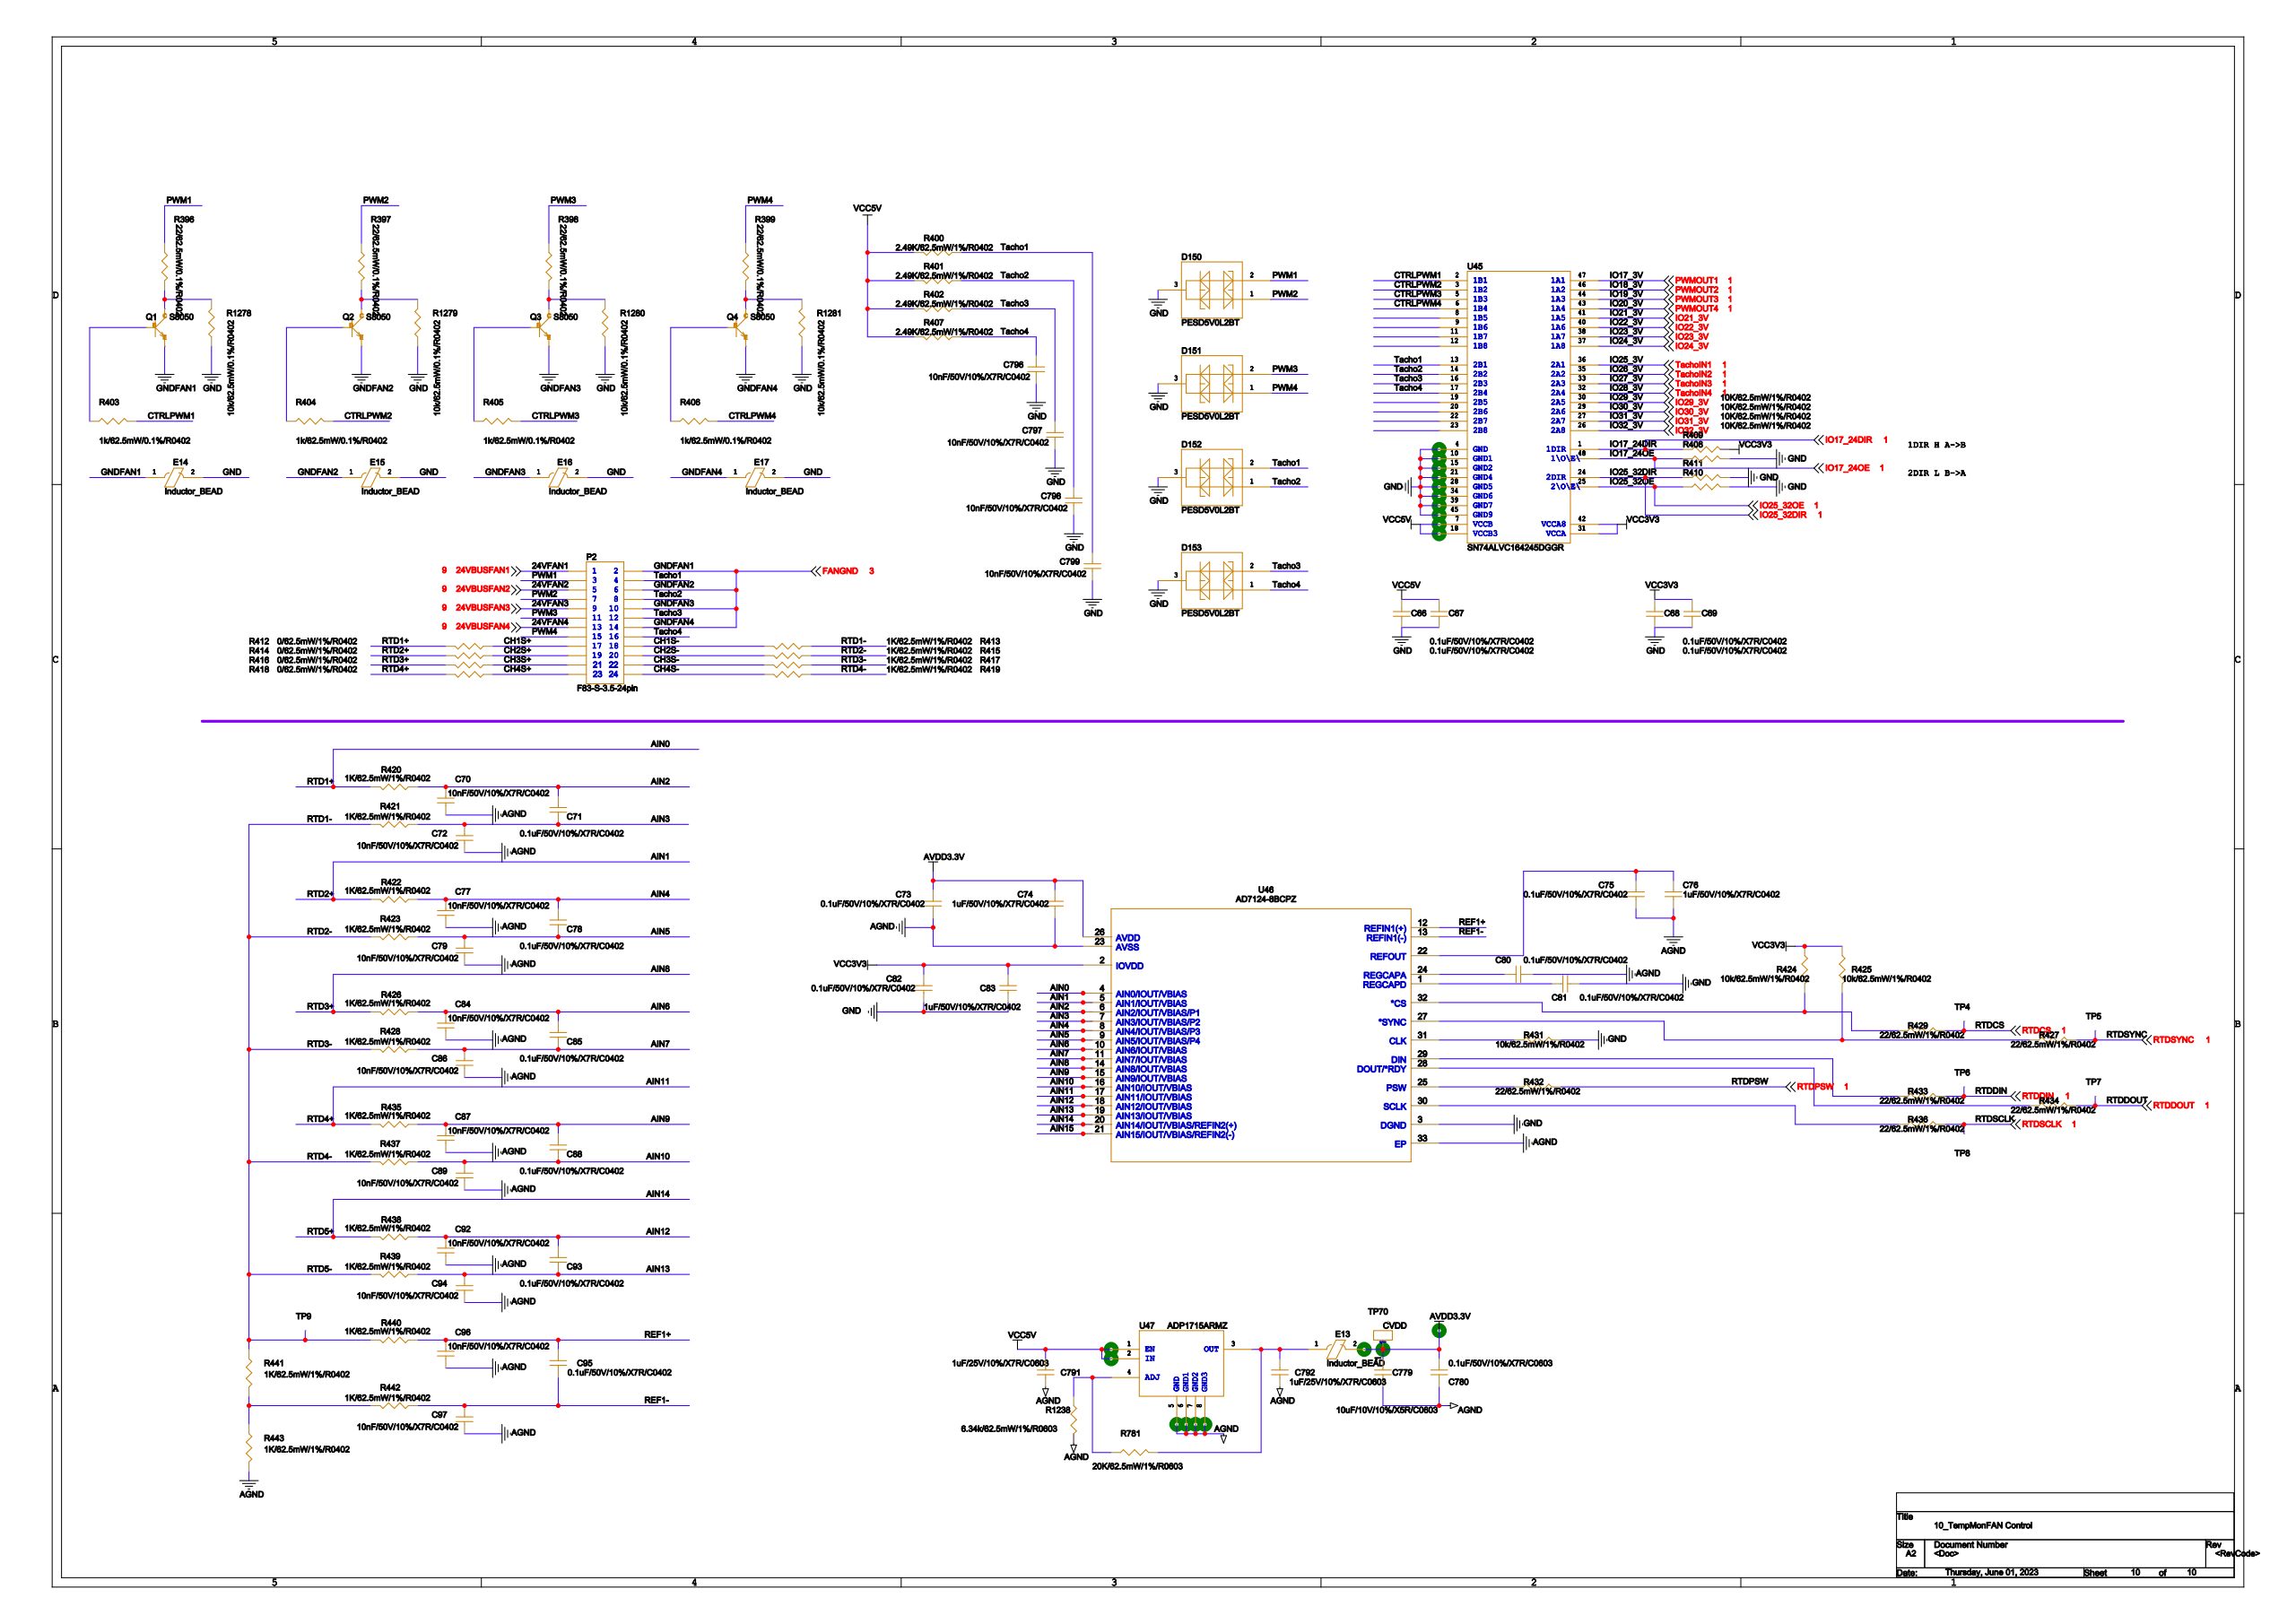Circuit board | Cadence Allegro | 480 parts | 625 nets | one sheet of the schematic
Parts on this sheet (reference | value | footprint):
C66 | 0.1uF/50V/10%/X7R/C0402 | 0402
C67 | 0.1uF/50V/10%/X7R/C0402 | 0402
C68 | 0.1uF/50V/10%/X7R/C0402 | 0402
C69 | 0.1uF/50V/10%/X7R/C0402 | 0402
C70 | 10nF/50V/10%/X7R/C0402 | 0402
C71 | 0.1uF/50V/10%/X7R/C0402 | 0402
C72 | 10nF/50V/10%/X7R/C0402 | 0402
C73 | 0.1uF/50V/10%/X7R/C0402 | 0402
C74 | 1uF/50V/10%/X7R/C0402 | 0402
C75 | 0.1uF/50V/10%/X7R/C0402 | 0402
C76 | 1uF/50V/10%/X7R/C0402 | 0402
C77 | 10nF/50V/10%/X7R/C0402 | 0402
C78 | 0.1uF/50V/10%/X7R/C0402 | 0402
C79 | 10nF/50V/10%/X7R/C0402 | 0402
C80 | 0.1uF/50V/10%/X7R/C0402 | 0402
C81 | 0.1uF/50V/10%/X7R/C0402 | 0402
C82 | 0.1uF/50V/10%/X7R/C0402 | 0402
C83 | 1uF/50V/10%/X7R/C0402 | 0402
C84 | 10nF/50V/10%/X7R/C0402 | 0402
C85 | 0.1uF/50V/10%/X7R/C0402 | 0402
C86 | 10nF/50V/10%/X7R/C0402 | 0402
C87 | 10nF/50V/10%/X7R/C0402 | 0402
C88 | 0.1uF/50V/10%/X7R/C0402 | 0402
C89 | 10nF/50V/10%/X7R/C0402 | 0402
C92 | 10nF/50V/10%/X7R/C0402 | 0402
C93 | 0.1uF/50V/10%/X7R/C0402 | 0402
C94 | 10nF/50V/10%/X7R/C0402 | 0402
C95 | 0.1uF/50V/10%/X7R/C0402 | 0402
C96 | 10nF/50V/10%/X7R/C0402 | 0402
C97 | 10nF/50V/10%/X7R/C0402 | 0402
C779 | 10uF/10V/10%/X5R/C0603 | 0603C
C780 | 0.1uF/50V/10%/X7R/C0603 | 0603C
C791 | 1uF/25V/10%/X7R/C0603 | 0603C
C792 | 1uF/25V/10%/X7R/C0603 | 0603C
C796 | 10nF/50V/10%/X7R/C0402 | 0402
C797 | 10nF/50V/10%/X7R/C0402 | 0402
C798 | 10nF/50V/10%/X7R/C0402 | 0402
C799 | 10nF/50V/10%/X7R/C0402 | 0402
D150 | PESD5V0L2BT | SOT23
D151 | PESD5V0L2BT | SOT23
D152 | PESD5V0L2BT | SOT23
D153 | PESD5V0L2BT | SOT23
E13 | Inductor_BEAD | 0603R
E14 | Inductor_BEAD | 0603R
E15 | Inductor_BEAD | 0603R
E16 | Inductor_BEAD | 0603R
E17 | Inductor_BEAD | 0603R
P2 | F83-S-3.5-24pin | F83-S-3_5-24PIN
Q1 | S8050 | SOT-23
Q2 | S8050 | SOT-23
Q3 | S8050 | SOT-23
Q4 | S8050 | SOT-23
R396 | 22/62.5mW/0.1%/R0402 | 0402
R397 | 22/62.5mW/0.1%/R0402 | 0402
R398 | 22/62.5mW/0.1%/R0402 | 0402
R399 | 22/62.5mW/0.1%/R0402 | 0402
R400 | 2.49K/62.5mW/1%/R0402 | 0402
R401 | 2.49K/62.5mW/1%/R0402 | 0402
R402 | 2.49K/62.5mW/1%/R0402 | 0402
R403 | 1k/62.5mW/0.1%/R0402 | 0402
R404 | 1k/62.5mW/0.1%/R0402 | 0402
R405 | 1k/62.5mW/0.1%/R0402 | 0402
R406 | 1k/62.5mW/0.1%/R0402 | 0402
R407 | 2.49K/62.5mW/1%/R0402 | 0402
R408 | 10K/62.5mW/1%/R0402 | 0402
R409 | 10K/62.5mW/1%/R0402 | 0402
R410 | 10K/62.5mW/1%/R0402 | 0402
R411 | 10K/62.5mW/1%/R0402 | 0402
R412 | 0/62.5mW/1%/R0402 | 0402
R413 | 1K/62.5mW/1%/R0402 | 0402
R414 | 0/62.5mW/1%/R0402 | 0402
R415 | 1K/62.5mW/1%/R0402 | 0402
R416 | 0/62.5mW/1%/R0402 | 0402
R417 | 1K/62.5mW/1%/R0402 | 0402
R418 | 0/62.5mW/1%/R0402 | 0402
R419 | 1K/62.5mW/1%/R0402 | 0402
R420 | 1K/62.5mW/1%/R0402 | 0402
R421 | 1K/62.5mW/1%/R0402 | 0402
R422 | 1K/62.5mW/1%/R0402 | 0402
R423 | 1K/62.5mW/1%/R0402 | 0402
R424 | 10k/62.5mW/1%/R0402 | 0402
R425 | 10k/62.5mW/1%/R0402 | 0402
R426 | 1K/62.5mW/1%/R0402 | 0402
R427 | 22/62.5mW/1%/R0402 | 0402
R428 | 1K/62.5mW/1%/R0402 | 0402
R429 | 22/62.5mW/1%/R0402 | 0402
R431 | 10k/62.5mW/1%/R0402 | 0402
R432 | 22/62.5mW/1%/R0402 | 0402
R433 | 22/62.5mW/1%/R0402 | 0402
R434 | 22/62.5mW/1%/R0402 | 0402
R435 | 1K/62.5mW/1%/R0402 | 0402
R436 | 22/62.5mW/1%/R0402 | 0402
R437 | 1K/62.5mW/1%/R0402 | 0402
R438 | 1K/62.5mW/1%/R0402 | 0402
R439 | 1K/62.5mW/1%/R0402 | 0402
R440 | 1K/62.5mW/1%/R0402 | 0402
R441 | 1K/62.5mW/1%/R0402 | 0402
R442 | 1K/62.5mW/1%/R0402 | 0402
R443 | 1K/62.5mW/1%/R0402 | 0402
R781 | 20K/62.5mW/1%/R0603 | 0603R
R1238 | 6.34k/62.5mW/1%/R0603 | 0603R
R1278 | 10k/62.5mW/0.1%/R0402 | 0402
R1279 | 10k/62.5mW/0.1%/R0402 | 0402
R1280 | 10k/62.5mW/0.1%/R0402 | 0402
R1281 | 10k/62.5mW/0.1%/R0402 | 0402
TP4 | TEST POINT A | TEST_12MM
TP5 | TEST POINT A | TEST_12MM
TP6 | TEST POINT A | TEST_12MM
TP7 | TEST POINT A | TEST_12MM
TP8 | TEST POINT A | TEST_12MM
TP9 | TEST POINT A | TEST_12MM
TP70 | CVDD | D0_6
U45 | SN74ALVC164245DGGR | TSSOP-48
U46 | Value | CP_32_12_ADI
U47 | ADP1715ARMZ | MSOP8
Nets of these parts (net: part-pin ...):
AGND: C66-1 C67-1 C68-1 C69-1 C70-2 C72-2 C73-2 C74-2 C75-2 C76-2 C77-2 C79-2 C80-2 C81-2 C82-2 C83-2 C84-2 C86-2 C87-2 C89-2 C92-2 C94-2 C96-2 C97-2 C779-2 C780-2 C791-2 C792-2 C796-2 C797-2 C798-2 C799-2 D150-3 D151-3 D152-3 D153-3 E14-2 E15-2 E16-2 E17-2 R408-1 R410-1 R411-1 R431-2 R443-2 R1238-1 R1278-1 R1279-1 R1280-1 R1281-1 U47-5 U47-6 U47-7 U47-8 U45-4 U45-10 U45-15 U45-21 U45-28 U45-34 U45-39 U45-45 U46-3 U46-23 U46-33
N23420107: Q1-3 R396-2 R1278-2
N23420396: Q2-3 R397-2 R1279-2
N23420476: Q3-3 R398-2 R1280-2
N23420600: Q4-3 R399-2 R1281-2
N23420104: Q1-1 R403-1
CTRLPWM1: R403-2 U45-2
N23420393: Q2-1 R404-1
CTRLPWM2: R404-2 U45-3
N23420473: Q3-1 R405-1
CTRLPWM3: R405-2 U45-5
N23420597: Q4-1 R406-1
CTRLPWM4: R406-2 U45-6
BANK13_L7_N: R408-2 U45-48
BANK13_L3_N: R409-2 U45-1
3.3V: C68-2 C69-2 C82-1 C83-1 R409-1 R424-1 R425-1 U45-31 U45-42 U46-2
BANK13_L8_P: R432-2
BANK13_L9_P: R427-2 TP5-1
BANK13_IO0: R434-2 TP7-1
BANK13_L19_N: R433-2 TP6-1
BANK13_L20_N: R436-2 TP8-1
BANK13_L16_P: R429-2 TP4-1
BANK13_L24_N: R411-2 U45-24
BANK13_L18_P: R410-2 U45-25
VCC5V: C66-2 C67-2 C791-1 R400-2 R401-2 R402-2 R407-2 U47-1 U47-2 U45-7 U45-18
AVDD3.3V: C73-1 C74-1 C779-1 C780-1 E13-2 TP70-1 U46-26
N23528814: C792-1 E13-1 R781-1 U47-3
N23528786: R781-2 R1238-2 U47-4
24VBUSFAN1: P2-1
FANGND: E14-1 E15-1 E16-1 E17-1 Q1-2 Q2-2 Q3-2 Q4-2 P2-2 P2-6 P2-10 P2-14
PWM3: D151-2 R398-1 P2-11
TACHO3: C797-1 D153-2 R402-1 P2-12 U45-16
24VBUSFAN4: P2-13
PWM4: D151-1 R399-1 P2-15
TACHO4: C796-1 D153-1 R407-1 P2-16 U45-17
CH1S+: R412-1 P2-17
CH1S-: R413-2 P2-18
CH2S+: R414-1 P2-19
CH2S-: R415-2 P2-20
CH3S+: R416-1 P2-21
CH3S-: R417-2 P2-22
CH4S+: R418-1 P2-23
CH4S-: R419-2 P2-24
PWM1: D150-2 R396-1 P2-3
TACHO1: C799-1 D152-2 R400-1 P2-4 U45-13
24VBUSFAN2: P2-5
PWM2: D150-1 R397-1 P2-7
TACHO2: C798-1 D152-1 R401-1 P2-8 U45-14
24VBUSFAN3: P2-9
AIN2: C70-1 C71-1 R420-1 U46-6
AIN3: C71-2 C72-1 R421-1 U46-7
N23186471: C75-1 C76-1 U46-22
AIN4: C77-1 C78-1 R422-1 U46-8
AIN5: C78-2 C79-1 R423-1 U46-9
N23186180: C80-1 U46-24
N23186182: C81-1 U46-1
AIN6: C84-1 C85-1 R426-1 U46-10
AIN7: C85-2 C86-1 R428-1 U46-11
AIN9: C87-1 C88-1 R435-1 U46-15
AIN10: C88-2 C89-1 R437-1 U46-16
AIN12: C92-1 C93-1 R438-1 U46-18
AIN13: C93-2 C94-1 R439-1 U46-19
REF1+: C95-1 C96-1 R440-1 U46-12
REF1-: C95-2 C97-1 R442-1 U46-13
RTD1-: R413-1 R415-1 R417-1 R419-1 R421-2 R423-2 R428-2 R437-2 R439-2 R440-2 R441-1 TP9-1
AIN0: R412-2 R420-2 U46-4
AIN1: R414-2 R422-2 U46-5
AIN8: R416-2 R426-2 U46-14
AIN11: R418-2 R435-2 U46-17
AIN14: R438-2 U46-20
N23184433: R441-2 R442-2 R443-1
N23186319: R424-2 R429-1 U46-32
N23186325: R425-2 R427-1 U46-27
N23186239: R431-1 U46-31
N23186243: R432-1 U46-25
N23186381: R433-1 U46-29
N23186383: R434-1 U46-28
N23186389: R436-1 U46-30
IO21_3V: U45-41
IO22_3V: U45-40
IO23_3V: U45-38
IO24_3V: U45-37
IO29_3V: U45-30
IO30_3V: U45-29
IO31_3V: U45-27
IO32_3V: U45-26
AIN15: U46-21